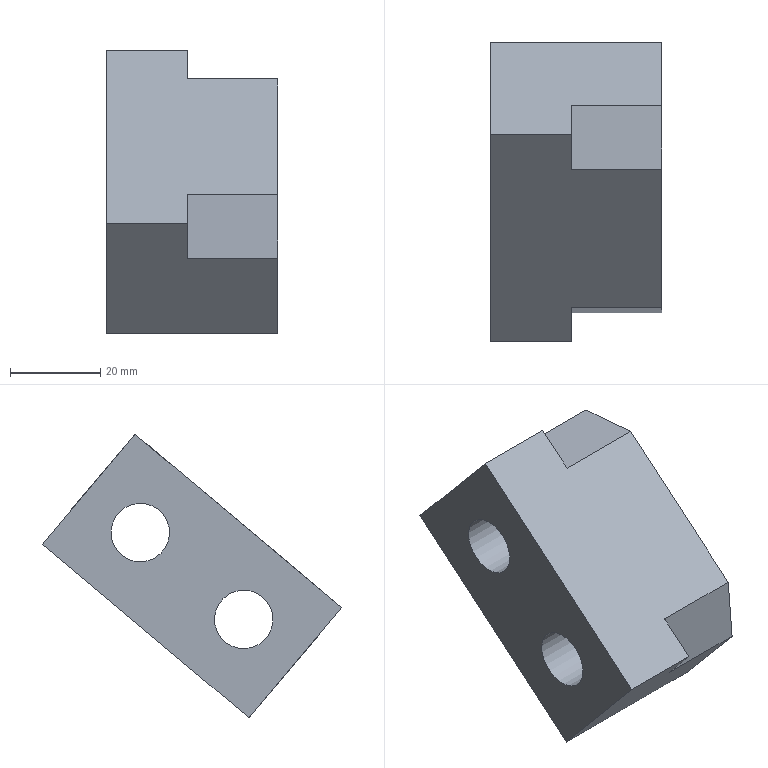Part | NX | features solid 2 | 1 solid | 16 faces | box 38 x 66.532 x 63.081 mm | volume 55430 mm3 | plane 12 | cylinder 4 | commonest cylinder face diameters 13 x2 20 x2
STEP:
#1=CARTESIAN_POINT('',(854.,-1105.608,-11.104));
#2=VERTEX_POINT('',#1);
#3=CARTESIAN_POINT('',(834.,-1105.608,-11.104));
#4=VERTEX_POINT('',#3);
#5=CARTESIAN_POINT('',(834.,-1105.608,-11.104));
#6=DIRECTION('',(1.,0.,0.));
#7=VECTOR('',#6,1000.);
#8=LINE('',#5,#7);
#9=EDGE_CURVE('',#2,#4,#8,.F.);
#10=ORIENTED_EDGE('',*,*,#9,.T.);
#11=CARTESIAN_POINT('',(834.,-1112.036,-3.444));
#12=VERTEX_POINT('',#11);
#13=CARTESIAN_POINT('',(834.,-1112.036,-3.444));
#14=DIRECTION('',(0.,0.6428,-0.766));
#15=VECTOR('',#14,1000.);
#16=LINE('',#13,#15);
#17=EDGE_CURVE('',#12,#4,#16,.T.);
#18=ORIENTED_EDGE('',*,*,#17,.F.);
#19=CARTESIAN_POINT('',(816.,-1112.036,-3.444));
#20=VERTEX_POINT('',#19);
#21=CARTESIAN_POINT('',(834.,-1112.036,-3.444));
#22=DIRECTION('',(1.,0.,0.));
#23=VECTOR('',#22,1000.);
#24=LINE('',#21,#23);
#25=EDGE_CURVE('',#12,#20,#24,.F.);
#26=ORIENTED_EDGE('',*,*,#25,.T.);
#27=CARTESIAN_POINT('',(816.,-1091.467,-27.957));
#28=VERTEX_POINT('',#27);
#29=CARTESIAN_POINT('',(816.,-1112.036,-3.444));
#30=DIRECTION('',(0.,-0.6428,0.766));
#31=VECTOR('',#30,1000.);
#32=LINE('',#29,#31);
#33=EDGE_CURVE('',#20,#28,#32,.F.);
#34=ORIENTED_EDGE('',*,*,#33,.T.);
#35=CARTESIAN_POINT('',(854.,-1091.467,-27.957));
#36=VERTEX_POINT('',#35);
#37=CARTESIAN_POINT('',(834.,-1091.467,-27.957));
#38=DIRECTION('',(1.,0.,0.));
#39=VECTOR('',#38,1000.);
#40=LINE('',#37,#39);
#41=EDGE_CURVE('',#36,#28,#40,.F.);
#42=ORIENTED_EDGE('',*,*,#41,.F.);
#43=CARTESIAN_POINT('',(854.,-1112.036,-3.444));
#44=DIRECTION('',(0.,-0.6428,0.766));
#45=VECTOR('',#44,1000.);
#46=LINE('',#43,#45);
#47=EDGE_CURVE('',#2,#36,#46,.F.);
#48=ORIENTED_EDGE('',*,*,#47,.F.);
#49=EDGE_LOOP('',(#10,#18,#26,#34,#42,#48));
#50=FACE_BOUND('',#49,.T.);
#51=CARTESIAN_POINT('',(834.,-1112.036,-3.444));
#52=DIRECTION('',(0.,-0.766,-0.6428));
#53=DIRECTION('',(0.,0.6428,-0.766));
#54=AXIS2_PLACEMENT_3D('',#51,#52,#53);
#55=PLANE('',#54);
#56=ADVANCED_FACE('',(#50),#55,.T.);
#57=ORIENTED_EDGE('',*,*,#41,.T.);
#58=CARTESIAN_POINT('',(816.,-1045.504,10.61));
#59=VERTEX_POINT('',#58);
#60=CARTESIAN_POINT('',(816.,-1091.467,-27.957));
#61=DIRECTION('',(0.,0.766,0.6428));
#62=VECTOR('',#61,1000.);
#63=LINE('',#60,#62);
#64=EDGE_CURVE('',#28,#59,#63,.T.);
#65=ORIENTED_EDGE('',*,*,#64,.T.);
#66=CARTESIAN_POINT('',(854.,-1045.504,10.61));
#67=VERTEX_POINT('',#66);
#68=CARTESIAN_POINT('',(834.,-1045.504,10.61));
#69=DIRECTION('',(1.,0.,0.));
#70=VECTOR('',#69,1000.);
#71=LINE('',#68,#70);
#72=EDGE_CURVE('',#67,#59,#71,.F.);
#73=ORIENTED_EDGE('',*,*,#72,.F.);
#74=CARTESIAN_POINT('',(854.,-1091.467,-27.957));
#75=DIRECTION('',(0.,0.766,0.6428));
#76=VECTOR('',#75,1000.);
#77=LINE('',#74,#76);
#78=EDGE_CURVE('',#36,#67,#77,.T.);
#79=ORIENTED_EDGE('',*,*,#78,.F.);
#80=EDGE_LOOP('',(#57,#65,#73,#79));
#81=FACE_BOUND('',#80,.T.);
#82=CARTESIAN_POINT('',(834.,-1091.467,-27.957));
#83=DIRECTION('',(0.,0.6428,-0.766));
#84=DIRECTION('',(0.,0.766,0.6428));
#85=AXIS2_PLACEMENT_3D('',#82,#83,#84);
#86=PLANE('',#85);
#87=ADVANCED_FACE('',(#81),#86,.T.);
#88=ORIENTED_EDGE('',*,*,#72,.T.);
#89=CARTESIAN_POINT('',(816.,-1066.074,35.123));
#90=VERTEX_POINT('',#89);
#91=CARTESIAN_POINT('',(816.,-1066.074,35.123));
#92=DIRECTION('',(0.,-0.6428,0.766));
#93=VECTOR('',#92,1000.);
#94=LINE('',#91,#93);
#95=EDGE_CURVE('',#90,#59,#94,.F.);
#96=ORIENTED_EDGE('',*,*,#95,.F.);
#97=CARTESIAN_POINT('',(834.,-1066.074,35.123));
#98=VERTEX_POINT('',#97);
#99=CARTESIAN_POINT('',(834.,-1066.074,35.123));
#100=DIRECTION('',(1.,0.,0.));
#101=VECTOR('',#100,1000.);
#102=LINE('',#99,#101);
#103=EDGE_CURVE('',#98,#90,#102,.F.);
#104=ORIENTED_EDGE('',*,*,#103,.F.);
#105=CARTESIAN_POINT('',(834.,-1059.646,27.463));
#106=VERTEX_POINT('',#105);
#107=CARTESIAN_POINT('',(834.,-1066.074,35.123));
#108=DIRECTION('',(0.,0.6428,-0.766));
#109=VECTOR('',#108,1000.);
#110=LINE('',#107,#109);
#111=EDGE_CURVE('',#98,#106,#110,.T.);
#112=ORIENTED_EDGE('',*,*,#111,.T.);
#113=CARTESIAN_POINT('',(854.,-1059.646,27.463));
#114=VERTEX_POINT('',#113);
#115=CARTESIAN_POINT('',(834.,-1059.646,27.463));
#116=DIRECTION('',(1.,0.,0.));
#117=VECTOR('',#116,1000.);
#118=LINE('',#115,#117);
#119=EDGE_CURVE('',#106,#114,#118,.T.);
#120=ORIENTED_EDGE('',*,*,#119,.T.);
#121=CARTESIAN_POINT('',(854.,-1066.074,35.123));
#122=DIRECTION('',(0.,-0.6428,0.766));
#123=VECTOR('',#122,1000.);
#124=LINE('',#121,#123);
#125=EDGE_CURVE('',#114,#67,#124,.F.);
#126=ORIENTED_EDGE('',*,*,#125,.T.);
#127=EDGE_LOOP('',(#88,#96,#104,#112,#120,#126));
#128=FACE_BOUND('',#127,.T.);
#129=CARTESIAN_POINT('',(834.,-1066.074,35.123));
#130=DIRECTION('',(0.,-0.766,-0.6428));
#131=DIRECTION('',(0.,0.6428,-0.766));
#132=AXIS2_PLACEMENT_3D('',#129,#130,#131);
#133=PLANE('',#132);
#134=ADVANCED_FACE('',(#128),#133,.F.);
#135=CARTESIAN_POINT('',(854.,-1073.734,28.696));
#136=VERTEX_POINT('',#135);
#137=CARTESIAN_POINT('',(834.,-1073.734,28.696));
#138=VERTEX_POINT('',#137);
#139=CARTESIAN_POINT('',(834.,-1073.734,28.696));
#140=DIRECTION('',(-1.,0.,0.));
#141=VECTOR('',#140,1000.);
#142=LINE('',#139,#141);
#143=EDGE_CURVE('',#136,#138,#142,.T.);
#144=ORIENTED_EDGE('',*,*,#143,.T.);
#145=CARTESIAN_POINT('',(834.,-1112.036,-3.444));
#146=DIRECTION('',(0.,0.766,0.6428));
#147=VECTOR('',#146,1000.);
#148=LINE('',#145,#147);
#149=EDGE_CURVE('',#138,#98,#148,.T.);
#150=ORIENTED_EDGE('',*,*,#149,.T.);
#151=ORIENTED_EDGE('',*,*,#103,.T.);
#152=CARTESIAN_POINT('',(816.,-1112.036,-3.444));
#153=DIRECTION('',(0.,0.766,0.6428));
#154=VECTOR('',#153,1000.);
#155=LINE('',#152,#154);
#156=EDGE_CURVE('',#20,#90,#155,.T.);
#157=ORIENTED_EDGE('',*,*,#156,.F.);
#158=ORIENTED_EDGE('',*,*,#25,.F.);
#159=CARTESIAN_POINT('',(834.,-1104.376,2.984));
#160=VERTEX_POINT('',#159);
#161=CARTESIAN_POINT('',(834.,-1112.036,-3.444));
#162=DIRECTION('',(0.,0.766,0.6428));
#163=VECTOR('',#162,1000.);
#164=LINE('',#161,#163);
#165=EDGE_CURVE('',#12,#160,#164,.T.);
#166=ORIENTED_EDGE('',*,*,#165,.T.);
#167=CARTESIAN_POINT('',(854.,-1104.376,2.984));
#168=VERTEX_POINT('',#167);
#169=CARTESIAN_POINT('',(834.,-1104.376,2.984));
#170=DIRECTION('',(1.,0.,0.));
#171=VECTOR('',#170,1000.);
#172=LINE('',#169,#171);
#173=EDGE_CURVE('',#160,#168,#172,.T.);
#174=ORIENTED_EDGE('',*,*,#173,.T.);
#175=CARTESIAN_POINT('',(854.,-1112.036,-3.444));
#176=DIRECTION('',(0.,0.766,0.6428));
#177=VECTOR('',#176,1000.);
#178=LINE('',#175,#177);
#179=EDGE_CURVE('',#168,#136,#178,.T.);
#180=ORIENTED_EDGE('',*,*,#179,.T.);
#181=EDGE_LOOP('',(#144,#150,#151,#157,#158,#166,#174,#180));
#182=FACE_BOUND('',#181,.T.);
#183=CARTESIAN_POINT('',(834.,-1112.036,-3.444));
#184=DIRECTION('',(0.,0.6428,-0.766));
#185=DIRECTION('',(0.,0.766,0.6428));
#186=AXIS2_PLACEMENT_3D('',#183,#184,#185);
#187=PLANE('',#186);
#188=ADVANCED_FACE('',(#182),#187,.F.);
#189=CARTESIAN_POINT('',(816.,-1068.408,19.626));
#190=VERTEX_POINT('',#189);
#191=CARTESIAN_POINT('',(816.,-1067.28,13.225));
#192=DIRECTION('',(1.,0.,0.));
#193=DIRECTION('',(0.,-0.1736,0.9848));
#194=AXIS2_PLACEMENT_3D('',#191,#192,#193);
#195=CIRCLE('',#194,6.5);
#196=EDGE_CURVE('',#190,#190,#195,.T.);
#197=ORIENTED_EDGE('',*,*,#196,.T.);
#198=EDGE_LOOP('',(#197));
#199=FACE_BOUND('',#198,.T.);
#200=CARTESIAN_POINT('',(816.,-1091.39,0.3426));
#201=VERTEX_POINT('',#200);
#202=CARTESIAN_POINT('',(816.,-1090.261,-6.059));
#203=DIRECTION('',(1.,0.,0.));
#204=DIRECTION('',(0.,-0.1736,0.9848));
#205=AXIS2_PLACEMENT_3D('',#202,#203,#204);
#206=CIRCLE('',#205,6.5);
#207=EDGE_CURVE('',#201,#201,#206,.T.);
#208=ORIENTED_EDGE('',*,*,#207,.T.);
#209=EDGE_LOOP('',(#208));
#210=FACE_BOUND('',#209,.T.);
#211=ORIENTED_EDGE('',*,*,#156,.T.);
#212=ORIENTED_EDGE('',*,*,#95,.T.);
#213=ORIENTED_EDGE('',*,*,#64,.F.);
#214=ORIENTED_EDGE('',*,*,#33,.F.);
#215=EDGE_LOOP('',(#211,#212,#213,#214));
#216=FACE_BOUND('',#215,.T.);
#217=CARTESIAN_POINT('',(816.,-1112.036,-3.444));
#218=DIRECTION('',(1.,0.,0.));
#219=DIRECTION('',(0.,0.766,0.6428));
#220=AXIS2_PLACEMENT_3D('',#217,#218,#219);
#221=PLANE('',#220);
#222=ADVANCED_FACE('',(#199,#210,#216),#221,.F.);
#223=CARTESIAN_POINT('',(854.,-1074.94,6.797));
#224=VERTEX_POINT('',#223);
#225=CARTESIAN_POINT('',(854.,-1067.28,13.225));
#226=DIRECTION('',(-1.,0.,0.));
#227=DIRECTION('',(0.,-0.766,-0.6428));
#228=AXIS2_PLACEMENT_3D('',#225,#226,#227);
#229=CIRCLE('',#228,10.);
#230=EDGE_CURVE('',#224,#224,#229,.T.);
#231=ORIENTED_EDGE('',*,*,#230,.T.);
#232=EDGE_LOOP('',(#231));
#233=FACE_BOUND('',#232,.T.);
#234=CARTESIAN_POINT('',(854.,-1097.921,-12.487));
#235=VERTEX_POINT('',#234);
#236=CARTESIAN_POINT('',(854.,-1090.261,-6.059));
#237=DIRECTION('',(-1.,0.,0.));
#238=DIRECTION('',(0.,-0.766,-0.6428));
#239=AXIS2_PLACEMENT_3D('',#236,#237,#238);
#240=CIRCLE('',#239,10.);
#241=EDGE_CURVE('',#235,#235,#240,.T.);
#242=ORIENTED_EDGE('',*,*,#241,.T.);
#243=EDGE_LOOP('',(#242));
#244=FACE_BOUND('',#243,.T.);
#245=ORIENTED_EDGE('',*,*,#125,.F.);
#246=CARTESIAN_POINT('',(854.,-1108.955,31.777));
#247=DIRECTION('',(0.,0.9962,-0.08716));
#248=VECTOR('',#247,1000.);
#249=LINE('',#246,#248);
#250=EDGE_CURVE('',#114,#136,#249,.F.);
#251=ORIENTED_EDGE('',*,*,#250,.T.);
#252=ORIENTED_EDGE('',*,*,#179,.F.);
#253=CARTESIAN_POINT('',(854.,-1104.992,-4.06));
#254=DIRECTION('',(0.,-0.08716,-0.9962));
#255=VECTOR('',#254,1000.);
#256=LINE('',#253,#255);
#257=EDGE_CURVE('',#168,#2,#256,.T.);
#258=ORIENTED_EDGE('',*,*,#257,.T.);
#259=ORIENTED_EDGE('',*,*,#47,.T.);
#260=ORIENTED_EDGE('',*,*,#78,.T.);
#261=EDGE_LOOP('',(#245,#251,#252,#258,#259,#260));
#262=FACE_BOUND('',#261,.T.);
#263=CARTESIAN_POINT('',(854.,-1112.036,-3.444));
#264=DIRECTION('',(1.,0.,0.));
#265=DIRECTION('',(0.,0.766,0.6428));
#266=AXIS2_PLACEMENT_3D('',#263,#264,#265);
#267=PLANE('',#266);
#268=ADVANCED_FACE('',(#233,#244,#262),#267,.T.);
#269=CARTESIAN_POINT('',(834.,-1073.734,28.696));
#270=DIRECTION('',(0.,-0.9962,0.08716));
#271=VECTOR('',#270,1000.);
#272=LINE('',#269,#271);
#273=EDGE_CURVE('',#138,#106,#272,.F.);
#274=ORIENTED_EDGE('',*,*,#273,.F.);
#275=ORIENTED_EDGE('',*,*,#143,.F.);
#276=ORIENTED_EDGE('',*,*,#250,.F.);
#277=ORIENTED_EDGE('',*,*,#119,.F.);
#278=EDGE_LOOP('',(#274,#275,#276,#277));
#279=FACE_BOUND('',#278,.T.);
#280=CARTESIAN_POINT('',(834.,-1073.734,28.696));
#281=DIRECTION('',(0.,-0.08716,-0.9962));
#282=DIRECTION('',(0.,0.9962,-0.08716));
#283=AXIS2_PLACEMENT_3D('',#280,#281,#282);
#284=PLANE('',#283);
#285=ADVANCED_FACE('',(#279),#284,.F.);
#286=CARTESIAN_POINT('',(834.,-1105.608,-11.104));
#287=DIRECTION('',(0.,0.08716,0.9962));
#288=VECTOR('',#287,1000.);
#289=LINE('',#286,#288);
#290=EDGE_CURVE('',#4,#160,#289,.T.);
#291=ORIENTED_EDGE('',*,*,#290,.F.);
#292=ORIENTED_EDGE('',*,*,#9,.F.);
#293=ORIENTED_EDGE('',*,*,#257,.F.);
#294=ORIENTED_EDGE('',*,*,#173,.F.);
#295=EDGE_LOOP('',(#291,#292,#293,#294));
#296=FACE_BOUND('',#295,.T.);
#297=CARTESIAN_POINT('',(834.,-1105.608,-11.104));
#298=DIRECTION('',(0.,-0.9962,0.08716));
#299=DIRECTION('',(0.,-0.08716,-0.9962));
#300=AXIS2_PLACEMENT_3D('',#297,#298,#299);
#301=PLANE('',#300);
#302=ADVANCED_FACE('',(#296),#301,.T.);
#303=ORIENTED_EDGE('',*,*,#17,.T.);
#304=ORIENTED_EDGE('',*,*,#290,.T.);
#305=ORIENTED_EDGE('',*,*,#165,.F.);
#306=EDGE_LOOP('',(#303,#304,#305));
#307=FACE_BOUND('',#306,.T.);
#308=CARTESIAN_POINT('',(834.,-1112.036,-3.444));
#309=DIRECTION('',(1.,0.,0.));
#310=DIRECTION('',(0.,0.766,0.6428));
#311=AXIS2_PLACEMENT_3D('',#308,#309,#310);
#312=PLANE('',#311);
#313=ADVANCED_FACE('',(#307),#312,.T.);
#314=ORIENTED_EDGE('',*,*,#149,.F.);
#315=ORIENTED_EDGE('',*,*,#273,.T.);
#316=ORIENTED_EDGE('',*,*,#111,.F.);
#317=EDGE_LOOP('',(#314,#315,#316));
#318=FACE_BOUND('',#317,.T.);
#319=CARTESIAN_POINT('',(834.,-1112.036,-3.444));
#320=DIRECTION('',(1.,0.,0.));
#321=DIRECTION('',(0.,0.766,0.6428));
#322=AXIS2_PLACEMENT_3D('',#319,#320,#321);
#323=PLANE('',#322);
#324=ADVANCED_FACE('',(#318),#323,.T.);
#325=CARTESIAN_POINT('',(839.,-1089.132,-12.46));
#326=VERTEX_POINT('',#325);
#327=CARTESIAN_POINT('',(839.,-1090.261,-6.059));
#328=DIRECTION('',(-1.,0.,0.));
#329=DIRECTION('',(0.,0.1736,-0.9848));
#330=AXIS2_PLACEMENT_3D('',#327,#328,#329);
#331=CIRCLE('',#330,6.5);
#332=EDGE_CURVE('',#326,#326,#331,.T.);
#333=ORIENTED_EDGE('',*,*,#332,.F.);
#334=EDGE_LOOP('',(#333));
#335=FACE_BOUND('',#334,.T.);
#336=ORIENTED_EDGE('',*,*,#207,.F.);
#337=EDGE_LOOP('',(#336));
#338=FACE_BOUND('',#337,.T.);
#339=CARTESIAN_POINT('',(-494165.984,-1090.261,-6.059));
#340=DIRECTION('',(-1.,0.,0.));
#341=DIRECTION('',(0.,-0.766,-0.6428));
#342=AXIS2_PLACEMENT_3D('',#339,#340,#341);
#343=CYLINDRICAL_SURFACE('',#342,6.5);
#344=ADVANCED_FACE('',(#335,#338),#343,.F.);
#345=ORIENTED_EDGE('',*,*,#332,.T.);
#346=EDGE_LOOP('',(#345));
#347=FACE_BOUND('',#346,.T.);
#348=CARTESIAN_POINT('',(839.,-1097.921,-12.487));
#349=VERTEX_POINT('',#348);
#350=CARTESIAN_POINT('',(839.,-1090.261,-6.059));
#351=DIRECTION('',(-1.,0.,0.));
#352=DIRECTION('',(0.,-0.766,-0.6428));
#353=AXIS2_PLACEMENT_3D('',#350,#351,#352);
#354=CIRCLE('',#353,10.);
#355=EDGE_CURVE('',#349,#349,#354,.T.);
#356=ORIENTED_EDGE('',*,*,#355,.F.);
#357=EDGE_LOOP('',(#356));
#358=FACE_BOUND('',#357,.T.);
#359=CARTESIAN_POINT('',(839.,-1090.261,-6.059));
#360=DIRECTION('',(-1.,0.,0.));
#361=DIRECTION('',(0.,-0.766,-0.6428));
#362=AXIS2_PLACEMENT_3D('',#359,#360,#361);
#363=PLANE('',#362);
#364=ADVANCED_FACE('',(#347,#358),#363,.F.);
#365=ORIENTED_EDGE('',*,*,#355,.T.);
#366=EDGE_LOOP('',(#365));
#367=FACE_BOUND('',#366,.T.);
#368=ORIENTED_EDGE('',*,*,#241,.F.);
#369=EDGE_LOOP('',(#368));
#370=FACE_BOUND('',#369,.T.);
#371=CARTESIAN_POINT('',(854.,-1090.261,-6.059));
#372=DIRECTION('',(-1.,0.,0.));
#373=DIRECTION('',(0.,-0.766,-0.6428));
#374=AXIS2_PLACEMENT_3D('',#371,#372,#373);
#375=CYLINDRICAL_SURFACE('',#374,10.);
#376=ADVANCED_FACE('',(#367,#370),#375,.F.);
#377=CARTESIAN_POINT('',(839.,-1066.151,6.824));
#378=VERTEX_POINT('',#377);
#379=CARTESIAN_POINT('',(839.,-1067.28,13.225));
#380=DIRECTION('',(-1.,0.,0.));
#381=DIRECTION('',(0.,0.1736,-0.9848));
#382=AXIS2_PLACEMENT_3D('',#379,#380,#381);
#383=CIRCLE('',#382,6.5);
#384=EDGE_CURVE('',#378,#378,#383,.T.);
#385=ORIENTED_EDGE('',*,*,#384,.F.);
#386=EDGE_LOOP('',(#385));
#387=FACE_BOUND('',#386,.T.);
#388=ORIENTED_EDGE('',*,*,#196,.F.);
#389=EDGE_LOOP('',(#388));
#390=FACE_BOUND('',#389,.T.);
#391=CARTESIAN_POINT('',(-494165.986,-1067.28,13.225));
#392=DIRECTION('',(-1.,0.,0.));
#393=DIRECTION('',(0.,-0.766,-0.6428));
#394=AXIS2_PLACEMENT_3D('',#391,#392,#393);
#395=CYLINDRICAL_SURFACE('',#394,6.5);
#396=ADVANCED_FACE('',(#387,#390),#395,.F.);
#397=ORIENTED_EDGE('',*,*,#384,.T.);
#398=EDGE_LOOP('',(#397));
#399=FACE_BOUND('',#398,.T.);
#400=CARTESIAN_POINT('',(839.,-1074.94,6.797));
#401=VERTEX_POINT('',#400);
#402=CARTESIAN_POINT('',(839.,-1067.28,13.225));
#403=DIRECTION('',(-1.,0.,0.));
#404=DIRECTION('',(0.,-0.766,-0.6428));
#405=AXIS2_PLACEMENT_3D('',#402,#403,#404);
#406=CIRCLE('',#405,10.);
#407=EDGE_CURVE('',#401,#401,#406,.T.);
#408=ORIENTED_EDGE('',*,*,#407,.F.);
#409=EDGE_LOOP('',(#408));
#410=FACE_BOUND('',#409,.T.);
#411=CARTESIAN_POINT('',(839.,-1067.28,13.225));
#412=DIRECTION('',(-1.,0.,0.));
#413=DIRECTION('',(0.,-0.766,-0.6428));
#414=AXIS2_PLACEMENT_3D('',#411,#412,#413);
#415=PLANE('',#414);
#416=ADVANCED_FACE('',(#399,#410),#415,.F.);
#417=ORIENTED_EDGE('',*,*,#407,.T.);
#418=EDGE_LOOP('',(#417));
#419=FACE_BOUND('',#418,.T.);
#420=ORIENTED_EDGE('',*,*,#230,.F.);
#421=EDGE_LOOP('',(#420));
#422=FACE_BOUND('',#421,.T.);
#423=CARTESIAN_POINT('',(854.,-1067.28,13.225));
#424=DIRECTION('',(-1.,0.,0.));
#425=DIRECTION('',(0.,-0.766,-0.6428));
#426=AXIS2_PLACEMENT_3D('',#423,#424,#425);
#427=CYLINDRICAL_SURFACE('',#426,10.);
#428=ADVANCED_FACE('',(#419,#422),#427,.F.);
#429=CLOSED_SHELL('',(#56,#87,#134,#188,#222,#268,#285,#302,#313,#324,#344,#364,#376,#396,#416,#428));
#430=MANIFOLD_SOLID_BREP('',#429);
#431=(LENGTH_UNIT()NAMED_UNIT(*)SI_UNIT(.MILLI.,.METRE.));
#432=UNCERTAINTY_MEASURE_WITH_UNIT(LENGTH_MEASURE(0.00001),#431,'','');
#433=(NAMED_UNIT(*)PLANE_ANGLE_UNIT()SI_UNIT($,.RADIAN.));
#434=(NAMED_UNIT(*)SI_UNIT($,.STERADIAN.)SOLID_ANGLE_UNIT());
#435=(GEOMETRIC_REPRESENTATION_CONTEXT(3)GLOBAL_UNCERTAINTY_ASSIGNED_CONTEXT((#432))GLOBAL_UNIT_ASSIGNED_CONTEXT((#431,#433,#434))REPRESENTATION_CONTEXT('',''));
#436=ADVANCED_BREP_SHAPE_REPRESENTATION('',(#430),#435);